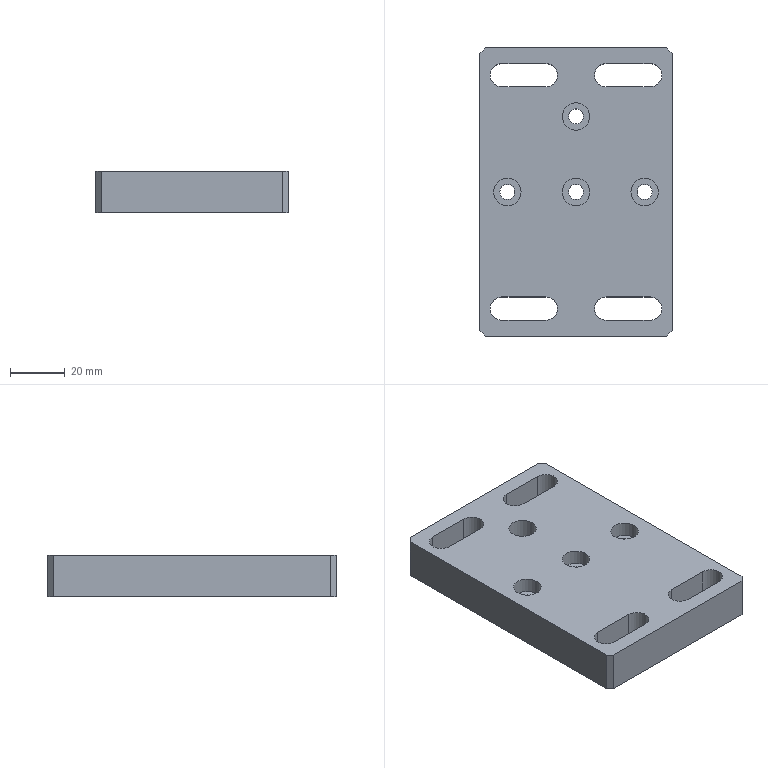Part | NX | 1 solid | 38 faces | box 70 x 105 x 15 mm | volume 95869 mm3 | plane 22 | cylinder 16 | commonest cylinder face diameters 8.5 x8 5.5 x4 10 x4
STEP:
#1=CARTESIAN_POINT('',(-20.,0.,9.6));
#2=VERTEX_POINT('',#1);
#3=CARTESIAN_POINT('',(-25.,0.,9.6));
#4=DIRECTION('',(0.,0.,1.));
#5=DIRECTION('',(1.,0.,0.));
#6=AXIS2_PLACEMENT_3D('',#3,#4,#5);
#7=CIRCLE('',#6,5.);
#8=EDGE_CURVE('',#2,#2,#7,.T.);
#9=ORIENTED_EDGE('',*,*,#8,.T.);
#10=EDGE_LOOP('',(#9));
#11=FACE_BOUND('',#10,.T.);
#12=CARTESIAN_POINT('',(-22.25,0.,9.6));
#13=VERTEX_POINT('',#12);
#14=CARTESIAN_POINT('',(-25.,0.,9.6));
#15=DIRECTION('',(0.,0.,1.));
#16=DIRECTION('',(1.,0.,0.));
#17=AXIS2_PLACEMENT_3D('',#14,#15,#16);
#18=CIRCLE('',#17,2.75);
#19=EDGE_CURVE('',#13,#13,#18,.T.);
#20=ORIENTED_EDGE('',*,*,#19,.F.);
#21=EDGE_LOOP('',(#20));
#22=FACE_BOUND('',#21,.T.);
#23=CARTESIAN_POINT('',(-22.25,0.,9.6));
#24=DIRECTION('',(0.,0.,-1.));
#25=DIRECTION('',(-1.,0.,0.));
#26=AXIS2_PLACEMENT_3D('',#23,#24,#25);
#27=PLANE('',#26);
#28=ADVANCED_FACE('',(#11,#22),#27,.F.);
#29=CARTESIAN_POINT('',(-5.,0.,9.6));
#30=VERTEX_POINT('',#29);
#31=CARTESIAN_POINT('',(0.,0.,9.6));
#32=DIRECTION('',(0.,0.,1.));
#33=DIRECTION('',(-1.,0.,0.));
#34=AXIS2_PLACEMENT_3D('',#31,#32,#33);
#35=CIRCLE('',#34,5.);
#36=EDGE_CURVE('',#30,#30,#35,.T.);
#37=ORIENTED_EDGE('',*,*,#36,.T.);
#38=EDGE_LOOP('',(#37));
#39=FACE_BOUND('',#38,.T.);
#40=CARTESIAN_POINT('',(-2.75,0.,9.6));
#41=VERTEX_POINT('',#40);
#42=CARTESIAN_POINT('',(0.,0.,9.6));
#43=DIRECTION('',(0.,0.,1.));
#44=DIRECTION('',(-1.,0.,0.));
#45=AXIS2_PLACEMENT_3D('',#42,#43,#44);
#46=CIRCLE('',#45,2.75);
#47=EDGE_CURVE('',#41,#41,#46,.T.);
#48=ORIENTED_EDGE('',*,*,#47,.F.);
#49=EDGE_LOOP('',(#48));
#50=FACE_BOUND('',#49,.T.);
#51=CARTESIAN_POINT('',(-22.25,0.,9.6));
#52=DIRECTION('',(0.,0.,-1.));
#53=DIRECTION('',(-1.,0.,0.));
#54=AXIS2_PLACEMENT_3D('',#51,#52,#53);
#55=PLANE('',#54);
#56=ADVANCED_FACE('',(#39,#50),#55,.F.);
#57=CARTESIAN_POINT('',(20.,0.,9.6));
#58=VERTEX_POINT('',#57);
#59=CARTESIAN_POINT('',(25.,0.,9.6));
#60=DIRECTION('',(0.,0.,1.));
#61=DIRECTION('',(-1.,0.,0.));
#62=AXIS2_PLACEMENT_3D('',#59,#60,#61);
#63=CIRCLE('',#62,5.);
#64=EDGE_CURVE('',#58,#58,#63,.T.);
#65=ORIENTED_EDGE('',*,*,#64,.T.);
#66=EDGE_LOOP('',(#65));
#67=FACE_BOUND('',#66,.T.);
#68=CARTESIAN_POINT('',(22.25,0.,9.6));
#69=VERTEX_POINT('',#68);
#70=CARTESIAN_POINT('',(25.,0.,9.6));
#71=DIRECTION('',(0.,0.,1.));
#72=DIRECTION('',(-1.,0.,0.));
#73=AXIS2_PLACEMENT_3D('',#70,#71,#72);
#74=CIRCLE('',#73,2.75);
#75=EDGE_CURVE('',#69,#69,#74,.T.);
#76=ORIENTED_EDGE('',*,*,#75,.F.);
#77=EDGE_LOOP('',(#76));
#78=FACE_BOUND('',#77,.T.);
#79=CARTESIAN_POINT('',(-22.25,0.,9.6));
#80=DIRECTION('',(0.,0.,-1.));
#81=DIRECTION('',(-1.,0.,0.));
#82=AXIS2_PLACEMENT_3D('',#79,#80,#81);
#83=PLANE('',#82);
#84=ADVANCED_FACE('',(#67,#78),#83,.F.);
#85=CARTESIAN_POINT('',(5.,27.5,8.));
#86=VERTEX_POINT('',#85);
#87=CARTESIAN_POINT('',(0.,27.5,8.));
#88=DIRECTION('',(0.,0.,1.));
#89=DIRECTION('',(1.,0.,0.));
#90=AXIS2_PLACEMENT_3D('',#87,#88,#89);
#91=CIRCLE('',#90,5.);
#92=EDGE_CURVE('',#86,#86,#91,.T.);
#93=ORIENTED_EDGE('',*,*,#92,.T.);
#94=EDGE_LOOP('',(#93));
#95=FACE_BOUND('',#94,.T.);
#96=CARTESIAN_POINT('',(2.75,27.5,8.));
#97=VERTEX_POINT('',#96);
#98=CARTESIAN_POINT('',(0.,27.5,8.));
#99=DIRECTION('',(0.,0.,1.));
#100=DIRECTION('',(1.,0.,0.));
#101=AXIS2_PLACEMENT_3D('',#98,#99,#100);
#102=CIRCLE('',#101,2.75);
#103=EDGE_CURVE('',#97,#97,#102,.T.);
#104=ORIENTED_EDGE('',*,*,#103,.F.);
#105=EDGE_LOOP('',(#104));
#106=FACE_BOUND('',#105,.T.);
#107=CARTESIAN_POINT('',(2.75,27.5,8.));
#108=DIRECTION('',(0.,0.,-1.));
#109=DIRECTION('',(-1.,0.,0.));
#110=AXIS2_PLACEMENT_3D('',#107,#108,#109);
#111=PLANE('',#110);
#112=ADVANCED_FACE('',(#95,#106),#111,.F.);
#113=CARTESIAN_POINT('',(-35.,-50.5,15.));
#114=VERTEX_POINT('',#113);
#115=CARTESIAN_POINT('',(-33.,-52.5,15.));
#116=VERTEX_POINT('',#115);
#117=CARTESIAN_POINT('',(-33.,-52.5,15.));
#118=DIRECTION('',(0.7071,-0.7071,0.));
#119=VECTOR('',#118,1000.);
#120=LINE('',#117,#119);
#121=EDGE_CURVE('',#114,#116,#120,.T.);
#122=ORIENTED_EDGE('',*,*,#121,.F.);
#123=CARTESIAN_POINT('',(-35.,-50.5,0.));
#124=VERTEX_POINT('',#123);
#125=CARTESIAN_POINT('',(-35.,-50.5,15.));
#126=DIRECTION('',(0.,0.,1.));
#127=VECTOR('',#126,1000.);
#128=LINE('',#125,#127);
#129=EDGE_CURVE('',#124,#114,#128,.T.);
#130=ORIENTED_EDGE('',*,*,#129,.F.);
#131=CARTESIAN_POINT('',(-33.,-52.5,0.));
#132=VERTEX_POINT('',#131);
#133=CARTESIAN_POINT('',(-42.75,-42.75,0.));
#134=DIRECTION('',(-0.7071,0.7071,0.));
#135=VECTOR('',#134,1000.);
#136=LINE('',#133,#135);
#137=EDGE_CURVE('',#132,#124,#136,.T.);
#138=ORIENTED_EDGE('',*,*,#137,.F.);
#139=CARTESIAN_POINT('',(-33.,-52.5,15.));
#140=DIRECTION('',(0.,0.,-1.));
#141=VECTOR('',#140,1000.);
#142=LINE('',#139,#141);
#143=EDGE_CURVE('',#116,#132,#142,.T.);
#144=ORIENTED_EDGE('',*,*,#143,.F.);
#145=EDGE_LOOP('',(#122,#130,#138,#144));
#146=FACE_BOUND('',#145,.T.);
#147=CARTESIAN_POINT('',(-33.,-52.5,15.));
#148=DIRECTION('',(0.7071,0.7071,0.));
#149=DIRECTION('',(0.,0.,-1.));
#150=AXIS2_PLACEMENT_3D('',#147,#148,#149);
#151=PLANE('',#150);
#152=ADVANCED_FACE('',(#146),#151,.F.);
#153=CARTESIAN_POINT('',(-33.,52.5,15.));
#154=VERTEX_POINT('',#153);
#155=CARTESIAN_POINT('',(-35.,50.5,15.));
#156=VERTEX_POINT('',#155);
#157=CARTESIAN_POINT('',(-35.,50.5,15.));
#158=DIRECTION('',(-0.7071,-0.7071,0.));
#159=VECTOR('',#158,1000.);
#160=LINE('',#157,#159);
#161=EDGE_CURVE('',#154,#156,#160,.T.);
#162=ORIENTED_EDGE('',*,*,#161,.F.);
#163=CARTESIAN_POINT('',(-33.,52.5,0.));
#164=VERTEX_POINT('',#163);
#165=CARTESIAN_POINT('',(-33.,52.5,15.));
#166=DIRECTION('',(0.,0.,1.));
#167=VECTOR('',#166,1000.);
#168=LINE('',#165,#167);
#169=EDGE_CURVE('',#164,#154,#168,.T.);
#170=ORIENTED_EDGE('',*,*,#169,.F.);
#171=CARTESIAN_POINT('',(-35.,50.5,0.));
#172=VERTEX_POINT('',#171);
#173=CARTESIAN_POINT('',(-42.75,42.75,0.));
#174=DIRECTION('',(0.7071,0.7071,0.));
#175=VECTOR('',#174,1000.);
#176=LINE('',#173,#175);
#177=EDGE_CURVE('',#172,#164,#176,.T.);
#178=ORIENTED_EDGE('',*,*,#177,.F.);
#179=CARTESIAN_POINT('',(-35.,50.5,15.));
#180=DIRECTION('',(0.,0.,-1.));
#181=VECTOR('',#180,1000.);
#182=LINE('',#179,#181);
#183=EDGE_CURVE('',#156,#172,#182,.T.);
#184=ORIENTED_EDGE('',*,*,#183,.F.);
#185=EDGE_LOOP('',(#162,#170,#178,#184));
#186=FACE_BOUND('',#185,.T.);
#187=CARTESIAN_POINT('',(-35.,50.5,15.));
#188=DIRECTION('',(0.7071,-0.7071,0.));
#189=DIRECTION('',(0.,0.,-1.));
#190=AXIS2_PLACEMENT_3D('',#187,#188,#189);
#191=PLANE('',#190);
#192=ADVANCED_FACE('',(#186),#191,.F.);
#193=CARTESIAN_POINT('',(33.,-52.5,15.));
#194=VERTEX_POINT('',#193);
#195=CARTESIAN_POINT('',(35.,-50.5,15.));
#196=VERTEX_POINT('',#195);
#197=CARTESIAN_POINT('',(35.,-50.5,15.));
#198=DIRECTION('',(0.7071,0.7071,0.));
#199=VECTOR('',#198,1000.);
#200=LINE('',#197,#199);
#201=EDGE_CURVE('',#194,#196,#200,.T.);
#202=ORIENTED_EDGE('',*,*,#201,.F.);
#203=CARTESIAN_POINT('',(33.,-52.5,0.));
#204=VERTEX_POINT('',#203);
#205=CARTESIAN_POINT('',(33.,-52.5,15.));
#206=DIRECTION('',(0.,0.,1.));
#207=VECTOR('',#206,1000.);
#208=LINE('',#205,#207);
#209=EDGE_CURVE('',#204,#194,#208,.T.);
#210=ORIENTED_EDGE('',*,*,#209,.F.);
#211=CARTESIAN_POINT('',(35.,-50.5,0.));
#212=VERTEX_POINT('',#211);
#213=CARTESIAN_POINT('',(42.75,-42.75,0.));
#214=DIRECTION('',(-0.7071,-0.7071,0.));
#215=VECTOR('',#214,1000.);
#216=LINE('',#213,#215);
#217=EDGE_CURVE('',#212,#204,#216,.T.);
#218=ORIENTED_EDGE('',*,*,#217,.F.);
#219=CARTESIAN_POINT('',(35.,-50.5,15.));
#220=DIRECTION('',(0.,0.,-1.));
#221=VECTOR('',#220,1000.);
#222=LINE('',#219,#221);
#223=EDGE_CURVE('',#196,#212,#222,.T.);
#224=ORIENTED_EDGE('',*,*,#223,.F.);
#225=EDGE_LOOP('',(#202,#210,#218,#224));
#226=FACE_BOUND('',#225,.T.);
#227=CARTESIAN_POINT('',(35.,-50.5,15.));
#228=DIRECTION('',(-0.7071,0.7071,0.));
#229=DIRECTION('',(0.,0.,-1.));
#230=AXIS2_PLACEMENT_3D('',#227,#228,#229);
#231=PLANE('',#230);
#232=ADVANCED_FACE('',(#226),#231,.F.);
#233=CARTESIAN_POINT('',(35.,50.5,15.));
#234=VERTEX_POINT('',#233);
#235=CARTESIAN_POINT('',(33.,52.5,15.));
#236=VERTEX_POINT('',#235);
#237=CARTESIAN_POINT('',(33.,52.5,15.));
#238=DIRECTION('',(-0.7071,0.7071,0.));
#239=VECTOR('',#238,1000.);
#240=LINE('',#237,#239);
#241=EDGE_CURVE('',#234,#236,#240,.T.);
#242=ORIENTED_EDGE('',*,*,#241,.F.);
#243=CARTESIAN_POINT('',(35.,50.5,0.));
#244=VERTEX_POINT('',#243);
#245=CARTESIAN_POINT('',(35.,50.5,15.));
#246=DIRECTION('',(0.,0.,1.));
#247=VECTOR('',#246,1000.);
#248=LINE('',#245,#247);
#249=EDGE_CURVE('',#244,#234,#248,.T.);
#250=ORIENTED_EDGE('',*,*,#249,.F.);
#251=CARTESIAN_POINT('',(33.,52.5,0.));
#252=VERTEX_POINT('',#251);
#253=CARTESIAN_POINT('',(42.75,42.75,0.));
#254=DIRECTION('',(0.7071,-0.7071,0.));
#255=VECTOR('',#254,1000.);
#256=LINE('',#253,#255);
#257=EDGE_CURVE('',#252,#244,#256,.T.);
#258=ORIENTED_EDGE('',*,*,#257,.F.);
#259=CARTESIAN_POINT('',(33.,52.5,15.));
#260=DIRECTION('',(0.,0.,-1.));
#261=VECTOR('',#260,1000.);
#262=LINE('',#259,#261);
#263=EDGE_CURVE('',#236,#252,#262,.T.);
#264=ORIENTED_EDGE('',*,*,#263,.F.);
#265=EDGE_LOOP('',(#242,#250,#258,#264));
#266=FACE_BOUND('',#265,.T.);
#267=CARTESIAN_POINT('',(33.,52.5,15.));
#268=DIRECTION('',(-0.7071,-0.7071,0.));
#269=DIRECTION('',(0.,0.,-1.));
#270=AXIS2_PLACEMENT_3D('',#267,#268,#269);
#271=PLANE('',#270);
#272=ADVANCED_FACE('',(#266),#271,.F.);
#273=CARTESIAN_POINT('',(-27.,46.75,15.));
#274=VERTEX_POINT('',#273);
#275=CARTESIAN_POINT('',(-27.,46.75,0.));
#276=VERTEX_POINT('',#275);
#277=CARTESIAN_POINT('',(-27.,46.75,30.));
#278=DIRECTION('',(0.,0.,-1.));
#279=VECTOR('',#278,1000.);
#280=LINE('',#277,#279);
#281=EDGE_CURVE('',#274,#276,#280,.T.);
#282=ORIENTED_EDGE('',*,*,#281,.T.);
#283=CARTESIAN_POINT('',(-11.,46.75,0.));
#284=VERTEX_POINT('',#283);
#285=CARTESIAN_POINT('',(-27.,46.75,0.));
#286=DIRECTION('',(1.,0.,0.));
#287=VECTOR('',#286,1000.);
#288=LINE('',#285,#287);
#289=EDGE_CURVE('',#276,#284,#288,.T.);
#290=ORIENTED_EDGE('',*,*,#289,.T.);
#291=CARTESIAN_POINT('',(-11.,46.75,15.));
#292=VERTEX_POINT('',#291);
#293=CARTESIAN_POINT('',(-11.,46.75,30.));
#294=DIRECTION('',(0.,0.,-1.));
#295=VECTOR('',#294,1000.);
#296=LINE('',#293,#295);
#297=EDGE_CURVE('',#292,#284,#296,.T.);
#298=ORIENTED_EDGE('',*,*,#297,.F.);
#299=CARTESIAN_POINT('',(0.,46.75,15.));
#300=DIRECTION('',(1.,0.,0.));
#301=VECTOR('',#300,1000.);
#302=LINE('',#299,#301);
#303=EDGE_CURVE('',#274,#292,#302,.T.);
#304=ORIENTED_EDGE('',*,*,#303,.F.);
#305=EDGE_LOOP('',(#282,#290,#298,#304));
#306=FACE_BOUND('',#305,.T.);
#307=CARTESIAN_POINT('',(-27.,46.75,30.));
#308=DIRECTION('',(0.,1.,0.));
#309=DIRECTION('',(-1.,0.,0.));
#310=AXIS2_PLACEMENT_3D('',#307,#308,#309);
#311=PLANE('',#310);
#312=ADVANCED_FACE('',(#306),#311,.F.);
#313=ORIENTED_EDGE('',*,*,#297,.T.);
#314=CARTESIAN_POINT('',(-11.,38.25,0.));
#315=VERTEX_POINT('',#314);
#316=CARTESIAN_POINT('',(-11.,42.5,0.));
#317=DIRECTION('',(0.,0.,-1.));
#318=DIRECTION('',(1.,0.,0.));
#319=AXIS2_PLACEMENT_3D('',#316,#317,#318);
#320=CIRCLE('',#319,4.25);
#321=EDGE_CURVE('',#284,#315,#320,.T.);
#322=ORIENTED_EDGE('',*,*,#321,.T.);
#323=CARTESIAN_POINT('',(-11.,38.25,15.));
#324=VERTEX_POINT('',#323);
#325=CARTESIAN_POINT('',(-11.,38.25,30.));
#326=DIRECTION('',(0.,0.,-1.));
#327=VECTOR('',#326,1000.);
#328=LINE('',#325,#327);
#329=EDGE_CURVE('',#324,#315,#328,.T.);
#330=ORIENTED_EDGE('',*,*,#329,.F.);
#331=CARTESIAN_POINT('',(-11.,42.5,15.));
#332=DIRECTION('',(0.,0.,-1.));
#333=DIRECTION('',(-1.,0.,0.));
#334=AXIS2_PLACEMENT_3D('',#331,#332,#333);
#335=CIRCLE('',#334,4.25);
#336=EDGE_CURVE('',#292,#324,#335,.T.);
#337=ORIENTED_EDGE('',*,*,#336,.F.);
#338=EDGE_LOOP('',(#313,#322,#330,#337));
#339=FACE_BOUND('',#338,.T.);
#340=CARTESIAN_POINT('',(-11.,42.5,30.));
#341=DIRECTION('',(0.,0.,-1.));
#342=DIRECTION('',(-1.,0.,0.));
#343=AXIS2_PLACEMENT_3D('',#340,#341,#342);
#344=CYLINDRICAL_SURFACE('',#343,4.25);
#345=ADVANCED_FACE('',(#339),#344,.F.);
#346=ORIENTED_EDGE('',*,*,#329,.T.);
#347=CARTESIAN_POINT('',(-27.,38.25,0.));
#348=VERTEX_POINT('',#347);
#349=CARTESIAN_POINT('',(-27.,38.25,0.));
#350=DIRECTION('',(-1.,0.,0.));
#351=VECTOR('',#350,1000.);
#352=LINE('',#349,#351);
#353=EDGE_CURVE('',#315,#348,#352,.T.);
#354=ORIENTED_EDGE('',*,*,#353,.T.);
#355=CARTESIAN_POINT('',(-27.,38.25,15.));
#356=VERTEX_POINT('',#355);
#357=CARTESIAN_POINT('',(-27.,38.25,30.));
#358=DIRECTION('',(0.,0.,-1.));
#359=VECTOR('',#358,1000.);
#360=LINE('',#357,#359);
#361=EDGE_CURVE('',#356,#348,#360,.T.);
#362=ORIENTED_EDGE('',*,*,#361,.F.);
#363=CARTESIAN_POINT('',(0.,38.25,15.));
#364=DIRECTION('',(-1.,0.,0.));
#365=VECTOR('',#364,1000.);
#366=LINE('',#363,#365);
#367=EDGE_CURVE('',#324,#356,#366,.T.);
#368=ORIENTED_EDGE('',*,*,#367,.F.);
#369=EDGE_LOOP('',(#346,#354,#362,#368));
#370=FACE_BOUND('',#369,.T.);
#371=CARTESIAN_POINT('',(-27.,38.25,30.));
#372=DIRECTION('',(0.,-1.,0.));
#373=DIRECTION('',(1.,0.,0.));
#374=AXIS2_PLACEMENT_3D('',#371,#372,#373);
#375=PLANE('',#374);
#376=ADVANCED_FACE('',(#370),#375,.F.);
#377=CARTESIAN_POINT('',(-27.,-38.25,15.));
#378=VERTEX_POINT('',#377);
#379=CARTESIAN_POINT('',(-27.,-38.25,0.));
#380=VERTEX_POINT('',#379);
#381=CARTESIAN_POINT('',(-27.,-38.25,30.));
#382=DIRECTION('',(0.,0.,-1.));
#383=VECTOR('',#382,1000.);
#384=LINE('',#381,#383);
#385=EDGE_CURVE('',#378,#380,#384,.T.);
#386=ORIENTED_EDGE('',*,*,#385,.T.);
#387=CARTESIAN_POINT('',(-11.,-38.25,0.));
#388=VERTEX_POINT('',#387);
#389=CARTESIAN_POINT('',(-27.,-38.25,0.));
#390=DIRECTION('',(1.,0.,0.));
#391=VECTOR('',#390,1000.);
#392=LINE('',#389,#391);
#393=EDGE_CURVE('',#380,#388,#392,.T.);
#394=ORIENTED_EDGE('',*,*,#393,.T.);
#395=CARTESIAN_POINT('',(-11.,-38.25,15.));
#396=VERTEX_POINT('',#395);
#397=CARTESIAN_POINT('',(-11.,-38.25,30.));
#398=DIRECTION('',(0.,0.,-1.));
#399=VECTOR('',#398,1000.);
#400=LINE('',#397,#399);
#401=EDGE_CURVE('',#396,#388,#400,.T.);
#402=ORIENTED_EDGE('',*,*,#401,.F.);
#403=CARTESIAN_POINT('',(0.,-38.25,15.));
#404=DIRECTION('',(1.,0.,0.));
#405=VECTOR('',#404,1000.);
#406=LINE('',#403,#405);
#407=EDGE_CURVE('',#378,#396,#406,.T.);
#408=ORIENTED_EDGE('',*,*,#407,.F.);
#409=EDGE_LOOP('',(#386,#394,#402,#408));
#410=FACE_BOUND('',#409,.T.);
#411=CARTESIAN_POINT('',(-27.,-38.25,30.));
#412=DIRECTION('',(0.,1.,0.));
#413=DIRECTION('',(-1.,0.,0.));
#414=AXIS2_PLACEMENT_3D('',#411,#412,#413);
#415=PLANE('',#414);
#416=ADVANCED_FACE('',(#410),#415,.F.);
#417=ORIENTED_EDGE('',*,*,#401,.T.);
#418=CARTESIAN_POINT('',(-11.,-46.75,0.));
#419=VERTEX_POINT('',#418);
#420=CARTESIAN_POINT('',(-11.,-42.5,0.));
#421=DIRECTION('',(0.,0.,-1.));
#422=DIRECTION('',(-1.,0.,0.));
#423=AXIS2_PLACEMENT_3D('',#420,#421,#422);
#424=CIRCLE('',#423,4.25);
#425=EDGE_CURVE('',#388,#419,#424,.T.);
#426=ORIENTED_EDGE('',*,*,#425,.T.);
#427=CARTESIAN_POINT('',(-11.,-46.75,15.));
#428=VERTEX_POINT('',#427);
#429=CARTESIAN_POINT('',(-11.,-46.75,30.));
#430=DIRECTION('',(0.,0.,-1.));
#431=VECTOR('',#430,1000.);
#432=LINE('',#429,#431);
#433=EDGE_CURVE('',#428,#419,#432,.T.);
#434=ORIENTED_EDGE('',*,*,#433,.F.);
#435=CARTESIAN_POINT('',(-11.,-42.5,15.));
#436=DIRECTION('',(0.,0.,-1.));
#437=DIRECTION('',(-1.,0.,0.));
#438=AXIS2_PLACEMENT_3D('',#435,#436,#437);
#439=CIRCLE('',#438,4.25);
#440=EDGE_CURVE('',#396,#428,#439,.T.);
#441=ORIENTED_EDGE('',*,*,#440,.F.);
#442=EDGE_LOOP('',(#417,#426,#434,#441));
#443=FACE_BOUND('',#442,.T.);
#444=CARTESIAN_POINT('',(-11.,-42.5,30.));
#445=DIRECTION('',(0.,0.,-1.));
#446=DIRECTION('',(-1.,0.,0.));
#447=AXIS2_PLACEMENT_3D('',#444,#445,#446);
#448=CYLINDRICAL_SURFACE('',#447,4.25);
#449=ADVANCED_FACE('',(#443),#448,.F.);
#450=ORIENTED_EDGE('',*,*,#433,.T.);
#451=CARTESIAN_POINT('',(-27.,-46.75,0.));
#452=VERTEX_POINT('',#451);
#453=CARTESIAN_POINT('',(-27.,-46.75,0.));
#454=DIRECTION('',(-1.,0.,0.));
#455=VECTOR('',#454,1000.);
#456=LINE('',#453,#455);
#457=EDGE_CURVE('',#419,#452,#456,.T.);
#458=ORIENTED_EDGE('',*,*,#457,.T.);
#459=CARTESIAN_POINT('',(-27.,-46.75,15.));
#460=VERTEX_POINT('',#459);
#461=CARTESIAN_POINT('',(-27.,-46.75,30.));
#462=DIRECTION('',(0.,0.,-1.));
#463=VECTOR('',#462,1000.);
#464=LINE('',#461,#463);
#465=EDGE_CURVE('',#460,#452,#464,.T.);
#466=ORIENTED_EDGE('',*,*,#465,.F.);
#467=CARTESIAN_POINT('',(0.,-46.75,15.));
#468=DIRECTION('',(-1.,0.,0.));
#469=VECTOR('',#468,1000.);
#470=LINE('',#467,#469);
#471=EDGE_CURVE('',#428,#460,#470,.T.);
#472=ORIENTED_EDGE('',*,*,#471,.F.);
#473=EDGE_LOOP('',(#450,#458,#466,#472));
#474=FACE_BOUND('',#473,.T.);
#475=CARTESIAN_POINT('',(-27.,-46.75,30.));
#476=DIRECTION('',(0.,-1.,0.));
#477=DIRECTION('',(1.,0.,0.));
#478=AXIS2_PLACEMENT_3D('',#475,#476,#477);
#479=PLANE('',#478);
#480=ADVANCED_FACE('',(#474),#479,.F.);
#481=CARTESIAN_POINT('',(27.,-46.75,15.));
#482=VERTEX_POINT('',#481);
#483=CARTESIAN_POINT('',(27.,-46.75,0.));
#484=VERTEX_POINT('',#483);
#485=CARTESIAN_POINT('',(27.,-46.75,30.));
#486=DIRECTION('',(0.,0.,-1.));
#487=VECTOR('',#486,1000.);
#488=LINE('',#485,#487);
#489=EDGE_CURVE('',#482,#484,#488,.T.);
#490=ORIENTED_EDGE('',*,*,#489,.T.);
#491=CARTESIAN_POINT('',(11.,-46.75,0.));
#492=VERTEX_POINT('',#491);
#493=CARTESIAN_POINT('',(-27.,-46.75,0.));
#494=DIRECTION('',(-1.,0.,0.));
#495=VECTOR('',#494,1000.);
#496=LINE('',#493,#495);
#497=EDGE_CURVE('',#484,#492,#496,.T.);
#498=ORIENTED_EDGE('',*,*,#497,.T.);
#499=CARTESIAN_POINT('',(11.,-46.75,15.));
#500=VERTEX_POINT('',#499);
#501=CARTESIAN_POINT('',(11.,-46.75,30.));
#502=DIRECTION('',(0.,0.,-1.));
#503=VECTOR('',#502,1000.);
#504=LINE('',#501,#503);
#505=EDGE_CURVE('',#500,#492,#504,.T.);
#506=ORIENTED_EDGE('',*,*,#505,.F.);
#507=CARTESIAN_POINT('',(0.,-46.75,15.));
#508=DIRECTION('',(-1.,0.,0.));
#509=VECTOR('',#508,1000.);
#510=LINE('',#507,#509);
#511=EDGE_CURVE('',#482,#500,#510,.T.);
#512=ORIENTED_EDGE('',*,*,#511,.F.);
#513=EDGE_LOOP('',(#490,#498,#506,#512));
#514=FACE_BOUND('',#513,.T.);
#515=CARTESIAN_POINT('',(-27.,-46.75,30.));
#516=DIRECTION('',(0.,-1.,0.));
#517=DIRECTION('',(1.,0.,0.));
#518=AXIS2_PLACEMENT_3D('',#515,#516,#517);
#519=PLANE('',#518);
#520=ADVANCED_FACE('',(#514),#519,.F.);
#521=CARTESIAN_POINT('',(11.,-38.25,15.));
#522=VERTEX_POINT('',#521);
#523=CARTESIAN_POINT('',(11.,-38.25,0.));
#524=VERTEX_POINT('',#523);
#525=CARTESIAN_POINT('',(11.,-38.25,30.));
#526=DIRECTION('',(0.,0.,-1.));
#527=VECTOR('',#526,1000.);
#528=LINE('',#525,#527);
#529=EDGE_CURVE('',#522,#524,#528,.T.);
#530=ORIENTED_EDGE('',*,*,#529,.T.);
#531=CARTESIAN_POINT('',(27.,-38.25,0.));
#532=VERTEX_POINT('',#531);
#533=CARTESIAN_POINT('',(-27.,-38.25,0.));
#534=DIRECTION('',(1.,0.,0.));
#535=VECTOR('',#534,1000.);
#536=LINE('',#533,#535);
#537=EDGE_CURVE('',#524,#532,#536,.T.);
#538=ORIENTED_EDGE('',*,*,#537,.T.);
#539=CARTESIAN_POINT('',(27.,-38.25,15.));
#540=VERTEX_POINT('',#539);
#541=CARTESIAN_POINT('',(27.,-38.25,30.));
#542=DIRECTION('',(0.,0.,-1.));
#543=VECTOR('',#542,1000.);
#544=LINE('',#541,#543);
#545=EDGE_CURVE('',#540,#532,#544,.T.);
#546=ORIENTED_EDGE('',*,*,#545,.F.);
#547=CARTESIAN_POINT('',(0.,-38.25,15.));
#548=DIRECTION('',(1.,0.,0.));
#549=VECTOR('',#548,1000.);
#550=LINE('',#547,#549);
#551=EDGE_CURVE('',#522,#540,#550,.T.);
#552=ORIENTED_EDGE('',*,*,#551,.F.);
#553=EDGE_LOOP('',(#530,#538,#546,#552));
#554=FACE_BOUND('',#553,.T.);
#555=CARTESIAN_POINT('',(-27.,-38.25,30.));
#556=DIRECTION('',(0.,1.,0.));
#557=DIRECTION('',(-1.,0.,0.));
#558=AXIS2_PLACEMENT_3D('',#555,#556,#557);
#559=PLANE('',#558);
#560=ADVANCED_FACE('',(#554),#559,.F.);
#561=ORIENTED_EDGE('',*,*,#545,.T.);
#562=CARTESIAN_POINT('',(27.,-42.5,0.));
#563=DIRECTION('',(0.,0.,-1.));
#564=DIRECTION('',(1.,0.,0.));
#565=AXIS2_PLACEMENT_3D('',#562,#563,#564);
#566=CIRCLE('',#565,4.25);
#567=EDGE_CURVE('',#532,#484,#566,.T.);
#568=ORIENTED_EDGE('',*,*,#567,.T.);
#569=ORIENTED_EDGE('',*,*,#489,.F.);
#570=CARTESIAN_POINT('',(27.,-42.5,15.));
#571=DIRECTION('',(0.,0.,-1.));
#572=DIRECTION('',(-1.,0.,0.));
#573=AXIS2_PLACEMENT_3D('',#570,#571,#572);
#574=CIRCLE('',#573,4.25);
#575=EDGE_CURVE('',#540,#482,#574,.T.);
#576=ORIENTED_EDGE('',*,*,#575,.F.);
#577=EDGE_LOOP('',(#561,#568,#569,#576));
#578=FACE_BOUND('',#577,.T.);
#579=CARTESIAN_POINT('',(27.,-42.5,30.));
#580=DIRECTION('',(0.,0.,-1.));
#581=DIRECTION('',(-1.,0.,0.));
#582=AXIS2_PLACEMENT_3D('',#579,#580,#581);
#583=CYLINDRICAL_SURFACE('',#582,4.25);
#584=ADVANCED_FACE('',(#578),#583,.F.);
#585=CARTESIAN_POINT('',(27.,38.25,15.));
#586=VERTEX_POINT('',#585);
#587=CARTESIAN_POINT('',(27.,38.25,0.));
#588=VERTEX_POINT('',#587);
#589=CARTESIAN_POINT('',(27.,38.25,30.));
#590=DIRECTION('',(0.,0.,-1.));
#591=VECTOR('',#590,1000.);
#592=LINE('',#589,#591);
#593=EDGE_CURVE('',#586,#588,#592,.T.);
#594=ORIENTED_EDGE('',*,*,#593,.T.);
#595=CARTESIAN_POINT('',(11.,38.25,0.));
#596=VERTEX_POINT('',#595);
#597=CARTESIAN_POINT('',(-27.,38.25,0.));
#598=DIRECTION('',(-1.,0.,0.));
#599=VECTOR('',#598,1000.);
#600=LINE('',#597,#599);
#601=EDGE_CURVE('',#588,#596,#600,.T.);
#602=ORIENTED_EDGE('',*,*,#601,.T.);
#603=CARTESIAN_POINT('',(11.,38.25,15.));
#604=VERTEX_POINT('',#603);
#605=CARTESIAN_POINT('',(11.,38.25,30.));
#606=DIRECTION('',(0.,0.,-1.));
#607=VECTOR('',#606,1000.);
#608=LINE('',#605,#607);
#609=EDGE_CURVE('',#604,#596,#608,.T.);
#610=ORIENTED_EDGE('',*,*,#609,.F.);
#611=CARTESIAN_POINT('',(0.,38.25,15.));
#612=DIRECTION('',(-1.,0.,0.));
#613=VECTOR('',#612,1000.);
#614=LINE('',#611,#613);
#615=EDGE_CURVE('',#586,#604,#614,.T.);
#616=ORIENTED_EDGE('',*,*,#615,.F.);
#617=EDGE_LOOP('',(#594,#602,#610,#616));
#618=FACE_BOUND('',#617,.T.);
#619=CARTESIAN_POINT('',(-27.,38.25,30.));
#620=DIRECTION('',(0.,-1.,0.));
#621=DIRECTION('',(1.,0.,0.));
#622=AXIS2_PLACEMENT_3D('',#619,#620,#621);
#623=PLANE('',#622);
#624=ADVANCED_FACE('',(#618),#623,.F.);
#625=CARTESIAN_POINT('',(11.,46.75,15.));
#626=VERTEX_POINT('',#625);
#627=CARTESIAN_POINT('',(11.,46.75,0.));
#628=VERTEX_POINT('',#627);
#629=CARTESIAN_POINT('',(11.,46.75,30.));
#630=DIRECTION('',(0.,0.,-1.));
#631=VECTOR('',#630,1000.);
#632=LINE('',#629,#631);
#633=EDGE_CURVE('',#626,#628,#632,.T.);
#634=ORIENTED_EDGE('',*,*,#633,.T.);
#635=CARTESIAN_POINT('',(27.,46.75,0.));
#636=VERTEX_POINT('',#635);
#637=CARTESIAN_POINT('',(-27.,46.75,0.));
#638=DIRECTION('',(1.,0.,0.));
#639=VECTOR('',#638,1000.);
#640=LINE('',#637,#639);
#641=EDGE_CURVE('',#628,#636,#640,.T.);
#642=ORIENTED_EDGE('',*,*,#641,.T.);
#643=CARTESIAN_POINT('',(27.,46.75,15.));
#644=VERTEX_POINT('',#643);
#645=CARTESIAN_POINT('',(27.,46.75,30.));
#646=DIRECTION('',(0.,0.,-1.));
#647=VECTOR('',#646,1000.);
#648=LINE('',#645,#647);
#649=EDGE_CURVE('',#644,#636,#648,.T.);
#650=ORIENTED_EDGE('',*,*,#649,.F.);
#651=CARTESIAN_POINT('',(0.,46.75,15.));
#652=DIRECTION('',(1.,0.,0.));
#653=VECTOR('',#652,1000.);
#654=LINE('',#651,#653);
#655=EDGE_CURVE('',#626,#644,#654,.T.);
#656=ORIENTED_EDGE('',*,*,#655,.F.);
#657=EDGE_LOOP('',(#634,#642,#650,#656));
#658=FACE_BOUND('',#657,.T.);
#659=CARTESIAN_POINT('',(-27.,46.75,30.));
#660=DIRECTION('',(0.,1.,0.));
#661=DIRECTION('',(-1.,0.,0.));
#662=AXIS2_PLACEMENT_3D('',#659,#660,#661);
#663=PLANE('',#662);
#664=ADVANCED_FACE('',(#658),#663,.F.);
#665=ORIENTED_EDGE('',*,*,#649,.T.);
#666=CARTESIAN_POINT('',(27.,42.5,0.));
#667=DIRECTION('',(0.,0.,-1.));
#668=DIRECTION('',(-1.,0.,0.));
#669=AXIS2_PLACEMENT_3D('',#666,#667,#668);
#670=CIRCLE('',#669,4.25);
#671=EDGE_CURVE('',#636,#588,#670,.T.);
#672=ORIENTED_EDGE('',*,*,#671,.T.);
#673=ORIENTED_EDGE('',*,*,#593,.F.);
#674=CARTESIAN_POINT('',(27.,42.5,15.));
#675=DIRECTION('',(0.,0.,-1.));
#676=DIRECTION('',(-1.,0.,0.));
#677=AXIS2_PLACEMENT_3D('',#674,#675,#676);
#678=CIRCLE('',#677,4.25);
#679=EDGE_CURVE('',#644,#586,#678,.T.);
#680=ORIENTED_EDGE('',*,*,#679,.F.);
#681=EDGE_LOOP('',(#665,#672,#673,#680));
#682=FACE_BOUND('',#681,.T.);
#683=CARTESIAN_POINT('',(27.,42.5,30.));
#684=DIRECTION('',(0.,0.,-1.));
#685=DIRECTION('',(-1.,0.,0.));
#686=AXIS2_PLACEMENT_3D('',#683,#684,#685);
#687=CYLINDRICAL_SURFACE('',#686,4.25);
#688=ADVANCED_FACE('',(#682),#687,.F.);
#689=CARTESIAN_POINT('',(-35.,52.5,0.));
#690=DIRECTION('',(-1.,0.,0.));
#691=VECTOR('',#690,1000.);
#692=LINE('',#689,#691);
#693=EDGE_CURVE('',#252,#164,#692,.T.);
#694=ORIENTED_EDGE('',*,*,#693,.F.);
#695=ORIENTED_EDGE('',*,*,#257,.T.);
#696=CARTESIAN_POINT('',(35.,-52.5,0.));
#697=DIRECTION('',(0.,1.,0.));
#698=VECTOR('',#697,1000.);
#699=LINE('',#696,#698);
#700=EDGE_CURVE('',#212,#244,#699,.T.);
#701=ORIENTED_EDGE('',*,*,#700,.F.);
#702=ORIENTED_EDGE('',*,*,#217,.T.);
#703=CARTESIAN_POINT('',(-35.,-52.5,0.));
#704=DIRECTION('',(1.,0.,0.));
#705=VECTOR('',#704,1000.);
#706=LINE('',#703,#705);
#707=EDGE_CURVE('',#132,#204,#706,.T.);
#708=ORIENTED_EDGE('',*,*,#707,.F.);
#709=ORIENTED_EDGE('',*,*,#137,.T.);
#710=CARTESIAN_POINT('',(-35.,-52.5,0.));
#711=DIRECTION('',(0.,-1.,0.));
#712=VECTOR('',#711,1000.);
#713=LINE('',#710,#712);
#714=EDGE_CURVE('',#172,#124,#713,.T.);
#715=ORIENTED_EDGE('',*,*,#714,.F.);
#716=ORIENTED_EDGE('',*,*,#177,.T.);
#717=EDGE_LOOP('',(#694,#695,#701,#702,#708,#709,#715,#716));
#718=FACE_BOUND('',#717,.T.);
#719=ORIENTED_EDGE('',*,*,#671,.F.);
#720=ORIENTED_EDGE('',*,*,#641,.F.);
#721=CARTESIAN_POINT('',(11.,42.5,0.));
#722=DIRECTION('',(0.,0.,-1.));
#723=DIRECTION('',(-1.,0.,0.));
#724=AXIS2_PLACEMENT_3D('',#721,#722,#723);
#725=CIRCLE('',#724,4.25);
#726=EDGE_CURVE('',#596,#628,#725,.T.);
#727=ORIENTED_EDGE('',*,*,#726,.F.);
#728=ORIENTED_EDGE('',*,*,#601,.F.);
#729=EDGE_LOOP('',(#719,#720,#727,#728));
#730=FACE_BOUND('',#729,.T.);
#731=ORIENTED_EDGE('',*,*,#567,.F.);
#732=ORIENTED_EDGE('',*,*,#537,.F.);
#733=CARTESIAN_POINT('',(11.,-42.5,0.));
#734=DIRECTION('',(0.,0.,-1.));
#735=DIRECTION('',(1.,0.,0.));
#736=AXIS2_PLACEMENT_3D('',#733,#734,#735);
#737=CIRCLE('',#736,4.25);
#738=EDGE_CURVE('',#492,#524,#737,.T.);
#739=ORIENTED_EDGE('',*,*,#738,.F.);
#740=ORIENTED_EDGE('',*,*,#497,.F.);
#741=EDGE_LOOP('',(#731,#732,#739,#740));
#742=FACE_BOUND('',#741,.T.);
#743=CARTESIAN_POINT('',(-27.,-42.5,0.));
#744=DIRECTION('',(0.,0.,-1.));
#745=DIRECTION('',(-1.,0.,0.));
#746=AXIS2_PLACEMENT_3D('',#743,#744,#745);
#747=CIRCLE('',#746,4.25);
#748=EDGE_CURVE('',#452,#380,#747,.T.);
#749=ORIENTED_EDGE('',*,*,#748,.F.);
#750=ORIENTED_EDGE('',*,*,#457,.F.);
#751=ORIENTED_EDGE('',*,*,#425,.F.);
#752=ORIENTED_EDGE('',*,*,#393,.F.);
#753=EDGE_LOOP('',(#749,#750,#751,#752));
#754=FACE_BOUND('',#753,.T.);
#755=CARTESIAN_POINT('',(-27.,42.5,0.));
#756=DIRECTION('',(0.,0.,-1.));
#757=DIRECTION('',(1.,0.,0.));
#758=AXIS2_PLACEMENT_3D('',#755,#756,#757);
#759=CIRCLE('',#758,4.25);
#760=EDGE_CURVE('',#348,#276,#759,.T.);
#761=ORIENTED_EDGE('',*,*,#760,.F.);
#762=ORIENTED_EDGE('',*,*,#353,.F.);
#763=ORIENTED_EDGE('',*,*,#321,.F.);
#764=ORIENTED_EDGE('',*,*,#289,.F.);
#765=EDGE_LOOP('',(#761,#762,#763,#764));
#766=FACE_BOUND('',#765,.T.);
#767=CARTESIAN_POINT('',(2.75,27.5,0.));
#768=VERTEX_POINT('',#767);
#769=CARTESIAN_POINT('',(0.,27.5,0.));
#770=DIRECTION('',(0.,0.,1.));
#771=DIRECTION('',(1.,0.,0.));
#772=AXIS2_PLACEMENT_3D('',#769,#770,#771);
#773=CIRCLE('',#772,2.75);
#774=EDGE_CURVE('',#768,#768,#773,.T.);
#775=ORIENTED_EDGE('',*,*,#774,.T.);
#776=EDGE_LOOP('',(#775));
#777=FACE_BOUND('',#776,.T.);
#778=CARTESIAN_POINT('',(27.75,0.,0.));
#779=VERTEX_POINT('',#778);
#780=CARTESIAN_POINT('',(25.,0.,0.));
#781=DIRECTION('',(0.,0.,1.));
#782=DIRECTION('',(1.,0.,0.));
#783=AXIS2_PLACEMENT_3D('',#780,#781,#782);
#784=CIRCLE('',#783,2.75);
#785=EDGE_CURVE('',#779,#779,#784,.T.);
#786=ORIENTED_EDGE('',*,*,#785,.T.);
#787=EDGE_LOOP('',(#786));
#788=FACE_BOUND('',#787,.T.);
#789=CARTESIAN_POINT('',(2.75,0.,0.));
#790=VERTEX_POINT('',#789);
#791=CARTESIAN_POINT('',(0.,0.,0.));
#792=DIRECTION('',(0.,0.,1.));
#793=DIRECTION('',(1.,0.,0.));
#794=AXIS2_PLACEMENT_3D('',#791,#792,#793);
#795=CIRCLE('',#794,2.75);
#796=EDGE_CURVE('',#790,#790,#795,.T.);
#797=ORIENTED_EDGE('',*,*,#796,.T.);
#798=EDGE_LOOP('',(#797));
#799=FACE_BOUND('',#798,.T.);
#800=CARTESIAN_POINT('',(-22.25,0.,0.));
#801=VERTEX_POINT('',#800);
#802=CARTESIAN_POINT('',(-25.,0.,0.));
#803=DIRECTION('',(0.,0.,1.));
#804=DIRECTION('',(1.,0.,0.));
#805=AXIS2_PLACEMENT_3D('',#802,#803,#804);
#806=CIRCLE('',#805,2.75);
#807=EDGE_CURVE('',#801,#801,#806,.T.);
#808=ORIENTED_EDGE('',*,*,#807,.T.);
#809=EDGE_LOOP('',(#808));
#810=FACE_BOUND('',#809,.T.);
#811=CARTESIAN_POINT('',(0.,0.,0.));
#812=DIRECTION('',(0.,0.,-1.));
#813=DIRECTION('',(-1.,0.,0.));
#814=AXIS2_PLACEMENT_3D('',#811,#812,#813);
#815=PLANE('',#814);
#816=ADVANCED_FACE('',(#718,#730,#742,#754,#766,#777,#788,#799,#810),#815,.T.);
#817=CARTESIAN_POINT('',(35.,-52.5,15.));
#818=DIRECTION('',(0.,1.,0.));
#819=VECTOR('',#818,1000.);
#820=LINE('',#817,#819);
#821=EDGE_CURVE('',#196,#234,#820,.T.);
#822=ORIENTED_EDGE('',*,*,#821,.T.);
#823=ORIENTED_EDGE('',*,*,#241,.T.);
#824=CARTESIAN_POINT('',(-35.,52.5,15.));
#825=DIRECTION('',(-1.,0.,0.));
#826=VECTOR('',#825,1000.);
#827=LINE('',#824,#826);
#828=EDGE_CURVE('',#236,#154,#827,.T.);
#829=ORIENTED_EDGE('',*,*,#828,.T.);
#830=ORIENTED_EDGE('',*,*,#161,.T.);
#831=CARTESIAN_POINT('',(-35.,-52.5,15.));
#832=DIRECTION('',(0.,-1.,0.));
#833=VECTOR('',#832,1000.);
#834=LINE('',#831,#833);
#835=EDGE_CURVE('',#156,#114,#834,.T.);
#836=ORIENTED_EDGE('',*,*,#835,.T.);
#837=ORIENTED_EDGE('',*,*,#121,.T.);
#838=CARTESIAN_POINT('',(-35.,-52.5,15.));
#839=DIRECTION('',(1.,0.,0.));
#840=VECTOR('',#839,1000.);
#841=LINE('',#838,#840);
#842=EDGE_CURVE('',#116,#194,#841,.T.);
#843=ORIENTED_EDGE('',*,*,#842,.T.);
#844=ORIENTED_EDGE('',*,*,#201,.T.);
#845=EDGE_LOOP('',(#822,#823,#829,#830,#836,#837,#843,#844));
#846=FACE_BOUND('',#845,.T.);
#847=ORIENTED_EDGE('',*,*,#655,.T.);
#848=ORIENTED_EDGE('',*,*,#679,.T.);
#849=ORIENTED_EDGE('',*,*,#615,.T.);
#850=CARTESIAN_POINT('',(11.,42.5,15.));
#851=DIRECTION('',(0.,0.,-1.));
#852=DIRECTION('',(-1.,0.,0.));
#853=AXIS2_PLACEMENT_3D('',#850,#851,#852);
#854=CIRCLE('',#853,4.25);
#855=EDGE_CURVE('',#604,#626,#854,.T.);
#856=ORIENTED_EDGE('',*,*,#855,.T.);
#857=EDGE_LOOP('',(#847,#848,#849,#856));
#858=FACE_BOUND('',#857,.T.);
#859=ORIENTED_EDGE('',*,*,#551,.T.);
#860=ORIENTED_EDGE('',*,*,#575,.T.);
#861=ORIENTED_EDGE('',*,*,#511,.T.);
#862=CARTESIAN_POINT('',(11.,-42.5,15.));
#863=DIRECTION('',(0.,0.,-1.));
#864=DIRECTION('',(-1.,0.,0.));
#865=AXIS2_PLACEMENT_3D('',#862,#863,#864);
#866=CIRCLE('',#865,4.25);
#867=EDGE_CURVE('',#500,#522,#866,.T.);
#868=ORIENTED_EDGE('',*,*,#867,.T.);
#869=EDGE_LOOP('',(#859,#860,#861,#868));
#870=FACE_BOUND('',#869,.T.);
#871=ORIENTED_EDGE('',*,*,#471,.T.);
#872=CARTESIAN_POINT('',(-27.,-42.5,15.));
#873=DIRECTION('',(0.,0.,-1.));
#874=DIRECTION('',(-1.,0.,0.));
#875=AXIS2_PLACEMENT_3D('',#872,#873,#874);
#876=CIRCLE('',#875,4.25);
#877=EDGE_CURVE('',#460,#378,#876,.T.);
#878=ORIENTED_EDGE('',*,*,#877,.T.);
#879=ORIENTED_EDGE('',*,*,#407,.T.);
#880=ORIENTED_EDGE('',*,*,#440,.T.);
#881=EDGE_LOOP('',(#871,#878,#879,#880));
#882=FACE_BOUND('',#881,.T.);
#883=ORIENTED_EDGE('',*,*,#367,.T.);
#884=CARTESIAN_POINT('',(-27.,42.5,15.));
#885=DIRECTION('',(0.,0.,-1.));
#886=DIRECTION('',(-1.,0.,0.));
#887=AXIS2_PLACEMENT_3D('',#884,#885,#886);
#888=CIRCLE('',#887,4.25);
#889=EDGE_CURVE('',#356,#274,#888,.T.);
#890=ORIENTED_EDGE('',*,*,#889,.T.);
#891=ORIENTED_EDGE('',*,*,#303,.T.);
#892=ORIENTED_EDGE('',*,*,#336,.T.);
#893=EDGE_LOOP('',(#883,#890,#891,#892));
#894=FACE_BOUND('',#893,.T.);
#895=CARTESIAN_POINT('',(5.,27.5,15.));
#896=VERTEX_POINT('',#895);
#897=CARTESIAN_POINT('',(0.,27.5,15.));
#898=DIRECTION('',(0.,0.,1.));
#899=DIRECTION('',(1.,0.,0.));
#900=AXIS2_PLACEMENT_3D('',#897,#898,#899);
#901=CIRCLE('',#900,5.);
#902=EDGE_CURVE('',#896,#896,#901,.T.);
#903=ORIENTED_EDGE('',*,*,#902,.F.);
#904=EDGE_LOOP('',(#903));
#905=FACE_BOUND('',#904,.T.);
#906=CARTESIAN_POINT('',(30.,0.,15.));
#907=VERTEX_POINT('',#906);
#908=CARTESIAN_POINT('',(25.,0.,15.));
#909=DIRECTION('',(0.,0.,1.));
#910=DIRECTION('',(1.,0.,0.));
#911=AXIS2_PLACEMENT_3D('',#908,#909,#910);
#912=CIRCLE('',#911,5.);
#913=EDGE_CURVE('',#907,#907,#912,.T.);
#914=ORIENTED_EDGE('',*,*,#913,.F.);
#915=EDGE_LOOP('',(#914));
#916=FACE_BOUND('',#915,.T.);
#917=CARTESIAN_POINT('',(5.,0.,15.));
#918=VERTEX_POINT('',#917);
#919=CARTESIAN_POINT('',(0.,0.,15.));
#920=DIRECTION('',(0.,0.,1.));
#921=DIRECTION('',(1.,0.,0.));
#922=AXIS2_PLACEMENT_3D('',#919,#920,#921);
#923=CIRCLE('',#922,5.);
#924=EDGE_CURVE('',#918,#918,#923,.T.);
#925=ORIENTED_EDGE('',*,*,#924,.F.);
#926=EDGE_LOOP('',(#925));
#927=FACE_BOUND('',#926,.T.);
#928=CARTESIAN_POINT('',(-20.,0.,15.));
#929=VERTEX_POINT('',#928);
#930=CARTESIAN_POINT('',(-25.,0.,15.));
#931=DIRECTION('',(0.,0.,1.));
#932=DIRECTION('',(1.,0.,0.));
#933=AXIS2_PLACEMENT_3D('',#930,#931,#932);
#934=CIRCLE('',#933,5.);
#935=EDGE_CURVE('',#929,#929,#934,.T.);
#936=ORIENTED_EDGE('',*,*,#935,.F.);
#937=EDGE_LOOP('',(#936));
#938=FACE_BOUND('',#937,.T.);
#939=CARTESIAN_POINT('',(0.,0.,15.));
#940=DIRECTION('',(0.,0.,-1.));
#941=DIRECTION('',(-1.,0.,0.));
#942=AXIS2_PLACEMENT_3D('',#939,#940,#941);
#943=PLANE('',#942);
#944=ADVANCED_FACE('',(#846,#858,#870,#882,#894,#905,#916,#927,#938),#943,.F.);
#945=ORIENTED_EDGE('',*,*,#707,.T.);
#946=ORIENTED_EDGE('',*,*,#209,.T.);
#947=ORIENTED_EDGE('',*,*,#842,.F.);
#948=ORIENTED_EDGE('',*,*,#143,.T.);
#949=EDGE_LOOP('',(#945,#946,#947,#948));
#950=FACE_BOUND('',#949,.T.);
#951=CARTESIAN_POINT('',(-35.,-52.5,15.));
#952=DIRECTION('',(0.,1.,0.));
#953=DIRECTION('',(0.,0.,1.));
#954=AXIS2_PLACEMENT_3D('',#951,#952,#953);
#955=PLANE('',#954);
#956=ADVANCED_FACE('',(#950),#955,.F.);
#957=ORIENTED_EDGE('',*,*,#835,.F.);
#958=ORIENTED_EDGE('',*,*,#183,.T.);
#959=ORIENTED_EDGE('',*,*,#714,.T.);
#960=ORIENTED_EDGE('',*,*,#129,.T.);
#961=EDGE_LOOP('',(#957,#958,#959,#960));
#962=FACE_BOUND('',#961,.T.);
#963=CARTESIAN_POINT('',(-35.,-52.5,15.));
#964=DIRECTION('',(1.,0.,0.));
#965=DIRECTION('',(0.,0.,-1.));
#966=AXIS2_PLACEMENT_3D('',#963,#964,#965);
#967=PLANE('',#966);
#968=ADVANCED_FACE('',(#962),#967,.F.);
#969=ORIENTED_EDGE('',*,*,#828,.F.);
#970=ORIENTED_EDGE('',*,*,#263,.T.);
#971=ORIENTED_EDGE('',*,*,#693,.T.);
#972=ORIENTED_EDGE('',*,*,#169,.T.);
#973=EDGE_LOOP('',(#969,#970,#971,#972));
#974=FACE_BOUND('',#973,.T.);
#975=CARTESIAN_POINT('',(-35.,52.5,15.));
#976=DIRECTION('',(0.,-1.,0.));
#977=DIRECTION('',(0.,0.,-1.));
#978=AXIS2_PLACEMENT_3D('',#975,#976,#977);
#979=PLANE('',#978);
#980=ADVANCED_FACE('',(#974),#979,.F.);
#981=ORIENTED_EDGE('',*,*,#700,.T.);
#982=ORIENTED_EDGE('',*,*,#249,.T.);
#983=ORIENTED_EDGE('',*,*,#821,.F.);
#984=ORIENTED_EDGE('',*,*,#223,.T.);
#985=EDGE_LOOP('',(#981,#982,#983,#984));
#986=FACE_BOUND('',#985,.T.);
#987=CARTESIAN_POINT('',(35.,-52.5,15.));
#988=DIRECTION('',(-1.,0.,0.));
#989=DIRECTION('',(0.,0.,1.));
#990=AXIS2_PLACEMENT_3D('',#987,#988,#989);
#991=PLANE('',#990);
#992=ADVANCED_FACE('',(#986),#991,.F.);
#993=ORIENTED_EDGE('',*,*,#855,.F.);
#994=ORIENTED_EDGE('',*,*,#609,.T.);
#995=ORIENTED_EDGE('',*,*,#726,.T.);
#996=ORIENTED_EDGE('',*,*,#633,.F.);
#997=EDGE_LOOP('',(#993,#994,#995,#996));
#998=FACE_BOUND('',#997,.T.);
#999=CARTESIAN_POINT('',(11.,42.5,30.));
#1000=DIRECTION('',(0.,0.,-1.));
#1001=DIRECTION('',(-1.,0.,0.));
#1002=AXIS2_PLACEMENT_3D('',#999,#1000,#1001);
#1003=CYLINDRICAL_SURFACE('',#1002,4.25);
#1004=ADVANCED_FACE('',(#998),#1003,.F.);
#1005=ORIENTED_EDGE('',*,*,#867,.F.);
#1006=ORIENTED_EDGE('',*,*,#505,.T.);
#1007=ORIENTED_EDGE('',*,*,#738,.T.);
#1008=ORIENTED_EDGE('',*,*,#529,.F.);
#1009=EDGE_LOOP('',(#1005,#1006,#1007,#1008));
#1010=FACE_BOUND('',#1009,.T.);
#1011=CARTESIAN_POINT('',(11.,-42.5,30.));
#1012=DIRECTION('',(0.,0.,-1.));
#1013=DIRECTION('',(-1.,0.,0.));
#1014=AXIS2_PLACEMENT_3D('',#1011,#1012,#1013);
#1015=CYLINDRICAL_SURFACE('',#1014,4.25);
#1016=ADVANCED_FACE('',(#1010),#1015,.F.);
#1017=ORIENTED_EDGE('',*,*,#877,.F.);
#1018=ORIENTED_EDGE('',*,*,#465,.T.);
#1019=ORIENTED_EDGE('',*,*,#748,.T.);
#1020=ORIENTED_EDGE('',*,*,#385,.F.);
#1021=EDGE_LOOP('',(#1017,#1018,#1019,#1020));
#1022=FACE_BOUND('',#1021,.T.);
#1023=CARTESIAN_POINT('',(-27.,-42.5,30.));
#1024=DIRECTION('',(0.,0.,-1.));
#1025=DIRECTION('',(-1.,0.,0.));
#1026=AXIS2_PLACEMENT_3D('',#1023,#1024,#1025);
#1027=CYLINDRICAL_SURFACE('',#1026,4.25);
#1028=ADVANCED_FACE('',(#1022),#1027,.F.);
#1029=ORIENTED_EDGE('',*,*,#889,.F.);
#1030=ORIENTED_EDGE('',*,*,#361,.T.);
#1031=ORIENTED_EDGE('',*,*,#760,.T.);
#1032=ORIENTED_EDGE('',*,*,#281,.F.);
#1033=EDGE_LOOP('',(#1029,#1030,#1031,#1032));
#1034=FACE_BOUND('',#1033,.T.);
#1035=CARTESIAN_POINT('',(-27.,42.5,30.));
#1036=DIRECTION('',(0.,0.,-1.));
#1037=DIRECTION('',(-1.,0.,0.));
#1038=AXIS2_PLACEMENT_3D('',#1035,#1036,#1037);
#1039=CYLINDRICAL_SURFACE('',#1038,4.25);
#1040=ADVANCED_FACE('',(#1034),#1039,.F.);
#1041=ORIENTED_EDGE('',*,*,#774,.F.);
#1042=EDGE_LOOP('',(#1041));
#1043=FACE_BOUND('',#1042,.T.);
#1044=ORIENTED_EDGE('',*,*,#103,.T.);
#1045=EDGE_LOOP('',(#1044));
#1046=FACE_BOUND('',#1045,.T.);
#1047=CARTESIAN_POINT('',(0.,27.5,15.));
#1048=DIRECTION('',(0.,0.,1.));
#1049=DIRECTION('',(1.,0.,0.));
#1050=AXIS2_PLACEMENT_3D('',#1047,#1048,#1049);
#1051=CYLINDRICAL_SURFACE('',#1050,2.75);
#1052=ADVANCED_FACE('',(#1043,#1046),#1051,.F.);
#1053=ORIENTED_EDGE('',*,*,#92,.F.);
#1054=EDGE_LOOP('',(#1053));
#1055=FACE_BOUND('',#1054,.T.);
#1056=ORIENTED_EDGE('',*,*,#902,.T.);
#1057=EDGE_LOOP('',(#1056));
#1058=FACE_BOUND('',#1057,.T.);
#1059=CARTESIAN_POINT('',(0.,27.5,15.));
#1060=DIRECTION('',(0.,0.,1.));
#1061=DIRECTION('',(1.,0.,0.));
#1062=AXIS2_PLACEMENT_3D('',#1059,#1060,#1061);
#1063=CYLINDRICAL_SURFACE('',#1062,5.);
#1064=ADVANCED_FACE('',(#1055,#1058),#1063,.F.);
#1065=ORIENTED_EDGE('',*,*,#785,.F.);
#1066=EDGE_LOOP('',(#1065));
#1067=FACE_BOUND('',#1066,.T.);
#1068=ORIENTED_EDGE('',*,*,#75,.T.);
#1069=EDGE_LOOP('',(#1068));
#1070=FACE_BOUND('',#1069,.T.);
#1071=CARTESIAN_POINT('',(25.,0.,15.));
#1072=DIRECTION('',(0.,0.,1.));
#1073=DIRECTION('',(1.,0.,0.));
#1074=AXIS2_PLACEMENT_3D('',#1071,#1072,#1073);
#1075=CYLINDRICAL_SURFACE('',#1074,2.75);
#1076=ADVANCED_FACE('',(#1067,#1070),#1075,.F.);
#1077=ORIENTED_EDGE('',*,*,#64,.F.);
#1078=EDGE_LOOP('',(#1077));
#1079=FACE_BOUND('',#1078,.T.);
#1080=ORIENTED_EDGE('',*,*,#913,.T.);
#1081=EDGE_LOOP('',(#1080));
#1082=FACE_BOUND('',#1081,.T.);
#1083=CARTESIAN_POINT('',(25.,0.,15.));
#1084=DIRECTION('',(0.,0.,1.));
#1085=DIRECTION('',(1.,0.,0.));
#1086=AXIS2_PLACEMENT_3D('',#1083,#1084,#1085);
#1087=CYLINDRICAL_SURFACE('',#1086,5.);
#1088=ADVANCED_FACE('',(#1079,#1082),#1087,.F.);
#1089=ORIENTED_EDGE('',*,*,#796,.F.);
#1090=EDGE_LOOP('',(#1089));
#1091=FACE_BOUND('',#1090,.T.);
#1092=ORIENTED_EDGE('',*,*,#47,.T.);
#1093=EDGE_LOOP('',(#1092));
#1094=FACE_BOUND('',#1093,.T.);
#1095=CARTESIAN_POINT('',(0.,0.,15.));
#1096=DIRECTION('',(0.,0.,1.));
#1097=DIRECTION('',(1.,0.,0.));
#1098=AXIS2_PLACEMENT_3D('',#1095,#1096,#1097);
#1099=CYLINDRICAL_SURFACE('',#1098,2.75);
#1100=ADVANCED_FACE('',(#1091,#1094),#1099,.F.);
#1101=ORIENTED_EDGE('',*,*,#36,.F.);
#1102=EDGE_LOOP('',(#1101));
#1103=FACE_BOUND('',#1102,.T.);
#1104=ORIENTED_EDGE('',*,*,#924,.T.);
#1105=EDGE_LOOP('',(#1104));
#1106=FACE_BOUND('',#1105,.T.);
#1107=CARTESIAN_POINT('',(0.,0.,15.));
#1108=DIRECTION('',(0.,0.,1.));
#1109=DIRECTION('',(1.,0.,0.));
#1110=AXIS2_PLACEMENT_3D('',#1107,#1108,#1109);
#1111=CYLINDRICAL_SURFACE('',#1110,5.);
#1112=ADVANCED_FACE('',(#1103,#1106),#1111,.F.);
#1113=ORIENTED_EDGE('',*,*,#807,.F.);
#1114=EDGE_LOOP('',(#1113));
#1115=FACE_BOUND('',#1114,.T.);
#1116=ORIENTED_EDGE('',*,*,#19,.T.);
#1117=EDGE_LOOP('',(#1116));
#1118=FACE_BOUND('',#1117,.T.);
#1119=CARTESIAN_POINT('',(-25.,0.,15.));
#1120=DIRECTION('',(0.,0.,1.));
#1121=DIRECTION('',(1.,0.,0.));
#1122=AXIS2_PLACEMENT_3D('',#1119,#1120,#1121);
#1123=CYLINDRICAL_SURFACE('',#1122,2.75);
#1124=ADVANCED_FACE('',(#1115,#1118),#1123,.F.);
#1125=ORIENTED_EDGE('',*,*,#8,.F.);
#1126=EDGE_LOOP('',(#1125));
#1127=FACE_BOUND('',#1126,.T.);
#1128=ORIENTED_EDGE('',*,*,#935,.T.);
#1129=EDGE_LOOP('',(#1128));
#1130=FACE_BOUND('',#1129,.T.);
#1131=CARTESIAN_POINT('',(-25.,0.,15.));
#1132=DIRECTION('',(0.,0.,1.));
#1133=DIRECTION('',(1.,0.,0.));
#1134=AXIS2_PLACEMENT_3D('',#1131,#1132,#1133);
#1135=CYLINDRICAL_SURFACE('',#1134,5.);
#1136=ADVANCED_FACE('',(#1127,#1130),#1135,.F.);
#1137=CLOSED_SHELL('',(#28,#56,#84,#112,#152,#192,#232,#272,#312,#345,#376,#416,#449,#480,#520,#560,#584,#624,#664,#688,#816,#944,#956,#968,#980,#992,#1004,#1016,#1028,#1040,#1052,#1064,#1076,#1088,#1100,#1112,#1124,#1136));
#1138=MANIFOLD_SOLID_BREP('',#1137);
#1139=(LENGTH_UNIT()NAMED_UNIT(*)SI_UNIT(.MILLI.,.METRE.));
#1140=UNCERTAINTY_MEASURE_WITH_UNIT(LENGTH_MEASURE(0.00001),#1139,'','');
#1141=(NAMED_UNIT(*)PLANE_ANGLE_UNIT()SI_UNIT($,.RADIAN.));
#1142=(NAMED_UNIT(*)SI_UNIT($,.STERADIAN.)SOLID_ANGLE_UNIT());
#1143=(GEOMETRIC_REPRESENTATION_CONTEXT(3)GLOBAL_UNCERTAINTY_ASSIGNED_CONTEXT((#1140))GLOBAL_UNIT_ASSIGNED_CONTEXT((#1139,#1141,#1142))REPRESENTATION_CONTEXT('',''));
#1144=ADVANCED_BREP_SHAPE_REPRESENTATION('',(#1138),#1143);